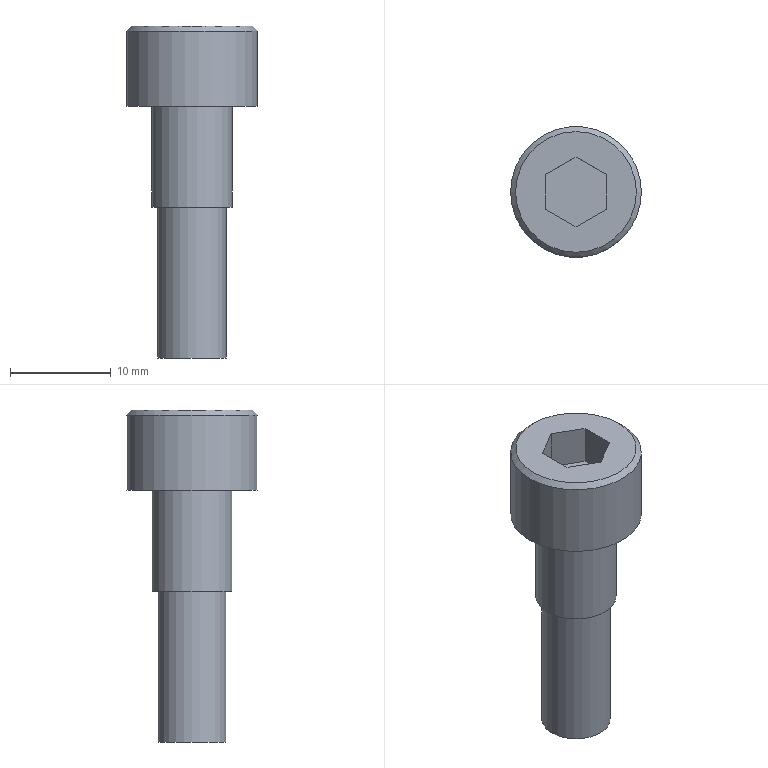Part | STEP file | M3-10_id62_x_t | 1 solid | 15 faces | box 13 x 13 x 33 mm | volume 1980 mm3 | plane 11 | cylinder 3 | cone 1 | commonest cylinder face diameters 6.8 x1 8 x1 13 x1
STEP:
#1=CARTESIAN_POINT('',(-245.9,-73.,-57.));
#2=VERTEX_POINT('',#1);
#3=CARTESIAN_POINT('',(-242.5,-73.,-57.));
#4=DIRECTION('',(0.,0.,-1.));
#5=DIRECTION('',(-1.,0.,0.));
#6=AXIS2_PLACEMENT_3D('',#3,#4,#5);
#7=CIRCLE('',#6,3.4);
#8=EDGE_CURVE('',#2,#2,#7,.T.);
#9=ORIENTED_EDGE('',*,*,#8,.F.);
#10=EDGE_LOOP('',(#9));
#11=FACE_BOUND('',#10,.T.);
#12=CARTESIAN_POINT('',(-238.5,-73.,-57.));
#13=VERTEX_POINT('',#12);
#14=CARTESIAN_POINT('',(-242.5,-73.,-57.));
#15=DIRECTION('',(0.,0.,1.));
#16=DIRECTION('',(1.,0.,0.));
#17=AXIS2_PLACEMENT_3D('',#14,#15,#16);
#18=CIRCLE('',#17,4.);
#19=EDGE_CURVE('',#13,#13,#18,.T.);
#20=ORIENTED_EDGE('',*,*,#19,.F.);
#21=EDGE_LOOP('',(#20));
#22=FACE_BOUND('',#21,.T.);
#23=CARTESIAN_POINT('',(-242.5,-73.,-57.));
#24=DIRECTION('',(0.,0.,-1.));
#25=DIRECTION('',(-1.,0.,0.));
#26=AXIS2_PLACEMENT_3D('',#23,#24,#25);
#27=PLANE('',#26);
#28=ADVANCED_FACE('',(#11,#22),#27,.T.);
#29=CARTESIAN_POINT('',(-246.5,-73.,-47.));
#30=VERTEX_POINT('',#29);
#31=CARTESIAN_POINT('',(-242.5,-73.,-47.));
#32=DIRECTION('',(0.,0.,1.));
#33=DIRECTION('',(-1.,0.,0.));
#34=AXIS2_PLACEMENT_3D('',#31,#32,#33);
#35=CIRCLE('',#34,4.);
#36=EDGE_CURVE('',#30,#30,#35,.T.);
#37=ORIENTED_EDGE('',*,*,#36,.F.);
#38=EDGE_LOOP('',(#37));
#39=FACE_BOUND('',#38,.T.);
#40=ORIENTED_EDGE('',*,*,#19,.T.);
#41=EDGE_LOOP('',(#40));
#42=FACE_BOUND('',#41,.T.);
#43=CARTESIAN_POINT('',(-242.5,-73.,-57.));
#44=DIRECTION('',(0.,0.,1.));
#45=DIRECTION('',(1.,0.,0.));
#46=AXIS2_PLACEMENT_3D('',#43,#44,#45);
#47=CYLINDRICAL_SURFACE('',#46,4.);
#48=ADVANCED_FACE('',(#39,#42),#47,.T.);
#49=CARTESIAN_POINT('',(-239.1,-73.,-72.));
#50=VERTEX_POINT('',#49);
#51=CARTESIAN_POINT('',(-242.5,-73.,-72.));
#52=DIRECTION('',(0.,0.,1.));
#53=DIRECTION('',(1.,0.,0.));
#54=AXIS2_PLACEMENT_3D('',#51,#52,#53);
#55=CIRCLE('',#54,3.4);
#56=EDGE_CURVE('',#50,#50,#55,.T.);
#57=ORIENTED_EDGE('',*,*,#56,.F.);
#58=EDGE_LOOP('',(#57));
#59=FACE_OUTER_BOUND('',#58,.T.);
#60=CARTESIAN_POINT('',(-242.5,-73.,-72.));
#61=DIRECTION('',(0.,0.,-1.));
#62=DIRECTION('',(-1.,0.,0.));
#63=AXIS2_PLACEMENT_3D('',#60,#61,#62);
#64=PLANE('',#63);
#65=ADVANCED_FACE('',(#59),#64,.T.);
#66=ORIENTED_EDGE('',*,*,#56,.T.);
#67=EDGE_LOOP('',(#66));
#68=FACE_BOUND('',#67,.T.);
#69=ORIENTED_EDGE('',*,*,#8,.T.);
#70=EDGE_LOOP('',(#69));
#71=FACE_BOUND('',#70,.T.);
#72=CARTESIAN_POINT('',(-242.5,-73.,-57.));
#73=DIRECTION('',(0.,0.,-1.));
#74=DIRECTION('',(1.,0.,0.));
#75=AXIS2_PLACEMENT_3D('',#72,#73,#74);
#76=CYLINDRICAL_SURFACE('',#75,3.4);
#77=ADVANCED_FACE('',(#68,#71),#76,.T.);
#78=CARTESIAN_POINT('',(-245.5,-71.268,-39.));
#79=VERTEX_POINT('',#78);
#80=CARTESIAN_POINT('',(-245.5,-74.732,-39.));
#81=VERTEX_POINT('',#80);
#82=CARTESIAN_POINT('',(-245.5,-71.268,-39.));
#83=DIRECTION('',(0.,-1.,0.));
#84=VECTOR('',#83,1.);
#85=LINE('',#82,#84);
#86=EDGE_CURVE('',#79,#81,#85,.T.);
#87=ORIENTED_EDGE('',*,*,#86,.F.);
#88=CARTESIAN_POINT('',(-242.5,-69.536,-39.));
#89=VERTEX_POINT('',#88);
#90=CARTESIAN_POINT('',(-242.5,-69.536,-39.));
#91=DIRECTION('',(-0.866,-0.5,0.));
#92=VECTOR('',#91,1.);
#93=LINE('',#90,#92);
#94=EDGE_CURVE('',#89,#79,#93,.T.);
#95=ORIENTED_EDGE('',*,*,#94,.F.);
#96=CARTESIAN_POINT('',(-239.5,-71.268,-39.));
#97=VERTEX_POINT('',#96);
#98=CARTESIAN_POINT('',(-239.5,-71.268,-39.));
#99=DIRECTION('',(-0.866,0.5,0.));
#100=VECTOR('',#99,1.);
#101=LINE('',#98,#100);
#102=EDGE_CURVE('',#97,#89,#101,.T.);
#103=ORIENTED_EDGE('',*,*,#102,.F.);
#104=CARTESIAN_POINT('',(-239.5,-74.732,-39.));
#105=VERTEX_POINT('',#104);
#106=CARTESIAN_POINT('',(-239.5,-74.732,-39.));
#107=DIRECTION('',(0.,1.,0.));
#108=VECTOR('',#107,1.);
#109=LINE('',#106,#108);
#110=EDGE_CURVE('',#105,#97,#109,.T.);
#111=ORIENTED_EDGE('',*,*,#110,.F.);
#112=CARTESIAN_POINT('',(-242.5,-76.464,-39.));
#113=VERTEX_POINT('',#112);
#114=CARTESIAN_POINT('',(-242.5,-76.464,-39.));
#115=DIRECTION('',(0.866,0.5,0.));
#116=VECTOR('',#115,1.);
#117=LINE('',#114,#116);
#118=EDGE_CURVE('',#113,#105,#117,.T.);
#119=ORIENTED_EDGE('',*,*,#118,.F.);
#120=CARTESIAN_POINT('',(-245.5,-74.732,-39.));
#121=DIRECTION('',(0.866,-0.5,0.));
#122=VECTOR('',#121,1.);
#123=LINE('',#120,#122);
#124=EDGE_CURVE('',#81,#113,#123,.T.);
#125=ORIENTED_EDGE('',*,*,#124,.F.);
#126=EDGE_LOOP('',(#87,#95,#103,#111,#119,#125));
#127=FACE_BOUND('',#126,.T.);
#128=CARTESIAN_POINT('',(-236.5,-73.,-39.));
#129=VERTEX_POINT('',#128);
#130=CARTESIAN_POINT('',(-242.5,-73.,-39.));
#131=DIRECTION('',(0.,0.,1.));
#132=DIRECTION('',(1.,0.,0.));
#133=AXIS2_PLACEMENT_3D('',#130,#131,#132);
#134=CIRCLE('',#133,6.);
#135=EDGE_CURVE('',#129,#129,#134,.T.);
#136=ORIENTED_EDGE('',*,*,#135,.T.);
#137=EDGE_LOOP('',(#136));
#138=FACE_BOUND('',#137,.T.);
#139=CARTESIAN_POINT('',(-242.5,-73.,-39.));
#140=DIRECTION('',(0.,0.,1.));
#141=DIRECTION('',(1.,0.,0.));
#142=AXIS2_PLACEMENT_3D('',#139,#140,#141);
#143=PLANE('',#142);
#144=ADVANCED_FACE('',(#127,#138),#143,.T.);
#145=ORIENTED_EDGE('',*,*,#36,.T.);
#146=EDGE_LOOP('',(#145));
#147=FACE_BOUND('',#146,.T.);
#148=CARTESIAN_POINT('',(-236.,-73.,-47.));
#149=VERTEX_POINT('',#148);
#150=CARTESIAN_POINT('',(-242.5,-73.,-47.));
#151=DIRECTION('',(0.,0.,1.));
#152=DIRECTION('',(1.,0.,0.));
#153=AXIS2_PLACEMENT_3D('',#150,#151,#152);
#154=CIRCLE('',#153,6.5);
#155=EDGE_CURVE('',#149,#149,#154,.T.);
#156=ORIENTED_EDGE('',*,*,#155,.F.);
#157=EDGE_LOOP('',(#156));
#158=FACE_BOUND('',#157,.T.);
#159=CARTESIAN_POINT('',(-242.5,-73.,-47.));
#160=DIRECTION('',(0.,0.,-1.));
#161=DIRECTION('',(-1.,0.,0.));
#162=AXIS2_PLACEMENT_3D('',#159,#160,#161);
#163=PLANE('',#162);
#164=ADVANCED_FACE('',(#147,#158),#163,.T.);
#165=CARTESIAN_POINT('',(-236.,-73.,-39.5));
#166=VERTEX_POINT('',#165);
#167=CARTESIAN_POINT('',(-242.5,-73.,-39.5));
#168=DIRECTION('',(0.,0.,-1.));
#169=DIRECTION('',(1.,0.,0.));
#170=AXIS2_PLACEMENT_3D('',#167,#168,#169);
#171=CIRCLE('',#170,6.5);
#172=EDGE_CURVE('',#166,#166,#171,.T.);
#173=ORIENTED_EDGE('',*,*,#172,.T.);
#174=EDGE_LOOP('',(#173));
#175=FACE_BOUND('',#174,.T.);
#176=ORIENTED_EDGE('',*,*,#155,.T.);
#177=EDGE_LOOP('',(#176));
#178=FACE_BOUND('',#177,.T.);
#179=CARTESIAN_POINT('',(-242.5,-73.,-47.));
#180=DIRECTION('',(0.,0.,1.));
#181=DIRECTION('',(1.,0.,0.));
#182=AXIS2_PLACEMENT_3D('',#179,#180,#181);
#183=CYLINDRICAL_SURFACE('',#182,6.5);
#184=ADVANCED_FACE('',(#175,#178),#183,.T.);
#185=ORIENTED_EDGE('',*,*,#135,.F.);
#186=EDGE_LOOP('',(#185));
#187=FACE_BOUND('',#186,.T.);
#188=ORIENTED_EDGE('',*,*,#172,.F.);
#189=EDGE_LOOP('',(#188));
#190=FACE_BOUND('',#189,.T.);
#191=CARTESIAN_POINT('',(-242.5,-73.,-39.5));
#192=DIRECTION('',(0.,0.,-1.));
#193=DIRECTION('',(-1.,0.,0.));
#194=AXIS2_PLACEMENT_3D('',#191,#192,#193);
#195=CONICAL_SURFACE('',#194,6.5,45.);
#196=ADVANCED_FACE('',(#187,#190),#195,.T.);
#197=ORIENTED_EDGE('',*,*,#86,.T.);
#198=CARTESIAN_POINT('',(-245.5,-74.732,-43.));
#199=VERTEX_POINT('',#198);
#200=CARTESIAN_POINT('',(-245.5,-74.732,-43.));
#201=DIRECTION('',(0.,0.,-1.));
#202=VECTOR('',#201,1.);
#203=LINE('',#200,#202);
#204=EDGE_CURVE('',#81,#199,#203,.T.);
#205=ORIENTED_EDGE('',*,*,#204,.T.);
#206=CARTESIAN_POINT('',(-245.5,-71.268,-43.));
#207=VERTEX_POINT('',#206);
#208=CARTESIAN_POINT('',(-245.5,-71.268,-43.));
#209=DIRECTION('',(0.,1.,0.));
#210=VECTOR('',#209,1.);
#211=LINE('',#208,#210);
#212=EDGE_CURVE('',#199,#207,#211,.T.);
#213=ORIENTED_EDGE('',*,*,#212,.T.);
#214=CARTESIAN_POINT('',(-245.5,-71.268,-43.));
#215=DIRECTION('',(0.,0.,-1.));
#216=VECTOR('',#215,1.);
#217=LINE('',#214,#216);
#218=EDGE_CURVE('',#79,#207,#217,.T.);
#219=ORIENTED_EDGE('',*,*,#218,.F.);
#220=EDGE_LOOP('',(#197,#205,#213,#219));
#221=FACE_OUTER_BOUND('',#220,.T.);
#222=CARTESIAN_POINT('',(-245.5,-71.268,-43.));
#223=DIRECTION('',(-1.,0.,0.));
#224=DIRECTION('',(0.,0.,1.));
#225=AXIS2_PLACEMENT_3D('',#222,#223,#224);
#226=PLANE('',#225);
#227=ADVANCED_FACE('',(#221),#226,.F.);
#228=ORIENTED_EDGE('',*,*,#124,.T.);
#229=CARTESIAN_POINT('',(-242.5,-76.464,-43.));
#230=VERTEX_POINT('',#229);
#231=CARTESIAN_POINT('',(-242.5,-76.464,-43.));
#232=DIRECTION('',(0.,0.,-1.));
#233=VECTOR('',#232,1.);
#234=LINE('',#231,#233);
#235=EDGE_CURVE('',#113,#230,#234,.T.);
#236=ORIENTED_EDGE('',*,*,#235,.T.);
#237=CARTESIAN_POINT('',(-245.5,-74.732,-43.));
#238=DIRECTION('',(-0.866,0.5,0.));
#239=VECTOR('',#238,1.);
#240=LINE('',#237,#239);
#241=EDGE_CURVE('',#230,#199,#240,.T.);
#242=ORIENTED_EDGE('',*,*,#241,.T.);
#243=ORIENTED_EDGE('',*,*,#204,.F.);
#244=EDGE_LOOP('',(#228,#236,#242,#243));
#245=FACE_OUTER_BOUND('',#244,.T.);
#246=CARTESIAN_POINT('',(-245.5,-74.732,-43.));
#247=DIRECTION('',(-0.5,-0.866,0.));
#248=DIRECTION('',(0.866,-0.5,0.));
#249=AXIS2_PLACEMENT_3D('',#246,#247,#248);
#250=PLANE('',#249);
#251=ADVANCED_FACE('',(#245),#250,.F.);
#252=ORIENTED_EDGE('',*,*,#118,.T.);
#253=CARTESIAN_POINT('',(-239.5,-74.732,-43.));
#254=VERTEX_POINT('',#253);
#255=CARTESIAN_POINT('',(-239.5,-74.732,-43.));
#256=DIRECTION('',(0.,0.,-1.));
#257=VECTOR('',#256,1.);
#258=LINE('',#255,#257);
#259=EDGE_CURVE('',#105,#254,#258,.T.);
#260=ORIENTED_EDGE('',*,*,#259,.T.);
#261=CARTESIAN_POINT('',(-242.5,-76.464,-43.));
#262=DIRECTION('',(-0.866,-0.5,0.));
#263=VECTOR('',#262,1.);
#264=LINE('',#261,#263);
#265=EDGE_CURVE('',#254,#230,#264,.T.);
#266=ORIENTED_EDGE('',*,*,#265,.T.);
#267=ORIENTED_EDGE('',*,*,#235,.F.);
#268=EDGE_LOOP('',(#252,#260,#266,#267));
#269=FACE_OUTER_BOUND('',#268,.T.);
#270=CARTESIAN_POINT('',(-242.5,-76.464,-43.));
#271=DIRECTION('',(0.5,-0.866,0.));
#272=DIRECTION('',(0.866,0.5,0.));
#273=AXIS2_PLACEMENT_3D('',#270,#271,#272);
#274=PLANE('',#273);
#275=ADVANCED_FACE('',(#269),#274,.F.);
#276=ORIENTED_EDGE('',*,*,#110,.T.);
#277=CARTESIAN_POINT('',(-239.5,-71.268,-43.));
#278=VERTEX_POINT('',#277);
#279=CARTESIAN_POINT('',(-239.5,-71.268,-43.));
#280=DIRECTION('',(0.,0.,-1.));
#281=VECTOR('',#280,1.);
#282=LINE('',#279,#281);
#283=EDGE_CURVE('',#97,#278,#282,.T.);
#284=ORIENTED_EDGE('',*,*,#283,.T.);
#285=CARTESIAN_POINT('',(-239.5,-74.732,-43.));
#286=DIRECTION('',(0.,-1.,0.));
#287=VECTOR('',#286,1.);
#288=LINE('',#285,#287);
#289=EDGE_CURVE('',#278,#254,#288,.T.);
#290=ORIENTED_EDGE('',*,*,#289,.T.);
#291=ORIENTED_EDGE('',*,*,#259,.F.);
#292=EDGE_LOOP('',(#276,#284,#290,#291));
#293=FACE_OUTER_BOUND('',#292,.T.);
#294=CARTESIAN_POINT('',(-239.5,-74.732,-43.));
#295=DIRECTION('',(1.,0.,0.));
#296=DIRECTION('',(0.,1.,0.));
#297=AXIS2_PLACEMENT_3D('',#294,#295,#296);
#298=PLANE('',#297);
#299=ADVANCED_FACE('',(#293),#298,.F.);
#300=ORIENTED_EDGE('',*,*,#102,.T.);
#301=CARTESIAN_POINT('',(-242.5,-69.536,-43.));
#302=VERTEX_POINT('',#301);
#303=CARTESIAN_POINT('',(-242.5,-69.536,-43.));
#304=DIRECTION('',(0.,0.,-1.));
#305=VECTOR('',#304,1.);
#306=LINE('',#303,#305);
#307=EDGE_CURVE('',#89,#302,#306,.T.);
#308=ORIENTED_EDGE('',*,*,#307,.T.);
#309=CARTESIAN_POINT('',(-239.5,-71.268,-43.));
#310=DIRECTION('',(0.866,-0.5,0.));
#311=VECTOR('',#310,1.);
#312=LINE('',#309,#311);
#313=EDGE_CURVE('',#302,#278,#312,.T.);
#314=ORIENTED_EDGE('',*,*,#313,.T.);
#315=ORIENTED_EDGE('',*,*,#283,.F.);
#316=EDGE_LOOP('',(#300,#308,#314,#315));
#317=FACE_OUTER_BOUND('',#316,.T.);
#318=CARTESIAN_POINT('',(-239.5,-71.268,-43.));
#319=DIRECTION('',(0.5,0.866,0.));
#320=DIRECTION('',(-0.866,0.5,0.));
#321=AXIS2_PLACEMENT_3D('',#318,#319,#320);
#322=PLANE('',#321);
#323=ADVANCED_FACE('',(#317),#322,.F.);
#324=ORIENTED_EDGE('',*,*,#94,.T.);
#325=ORIENTED_EDGE('',*,*,#218,.T.);
#326=CARTESIAN_POINT('',(-242.5,-69.536,-43.));
#327=DIRECTION('',(0.866,0.5,0.));
#328=VECTOR('',#327,1.);
#329=LINE('',#326,#328);
#330=EDGE_CURVE('',#207,#302,#329,.T.);
#331=ORIENTED_EDGE('',*,*,#330,.T.);
#332=ORIENTED_EDGE('',*,*,#307,.F.);
#333=EDGE_LOOP('',(#324,#325,#331,#332));
#334=FACE_OUTER_BOUND('',#333,.T.);
#335=CARTESIAN_POINT('',(-242.5,-69.536,-43.));
#336=DIRECTION('',(-0.5,0.866,0.));
#337=DIRECTION('',(-0.866,-0.5,0.));
#338=AXIS2_PLACEMENT_3D('',#335,#336,#337);
#339=PLANE('',#338);
#340=ADVANCED_FACE('',(#334),#339,.F.);
#341=ORIENTED_EDGE('',*,*,#212,.F.);
#342=ORIENTED_EDGE('',*,*,#241,.F.);
#343=ORIENTED_EDGE('',*,*,#265,.F.);
#344=ORIENTED_EDGE('',*,*,#289,.F.);
#345=ORIENTED_EDGE('',*,*,#313,.F.);
#346=ORIENTED_EDGE('',*,*,#330,.F.);
#347=EDGE_LOOP('',(#341,#342,#343,#344,#345,#346));
#348=FACE_OUTER_BOUND('',#347,.T.);
#349=CARTESIAN_POINT('',(-242.5,-73.,-43.));
#350=DIRECTION('',(0.,0.,1.));
#351=DIRECTION('',(1.,0.,0.));
#352=AXIS2_PLACEMENT_3D('',#349,#350,#351);
#353=PLANE('',#352);
#354=ADVANCED_FACE('',(#348),#353,.T.);
#355=CLOSED_SHELL('',(#28,#48,#65,#77,#144,#164,#184,#196,#227,#251,#275,#299,#323,#340,#354));
#356=MANIFOLD_SOLID_BREP('',#355);
#357=(LENGTH_UNIT()NAMED_UNIT(*)SI_UNIT(.MILLI.,.METRE.));
#358=UNCERTAINTY_MEASURE_WITH_UNIT(LENGTH_MEASURE(0.00002),#357,'','');
#359=(NAMED_UNIT(*)PLANE_ANGLE_UNIT()SI_UNIT($,.RADIAN.));
#360=PLANE_ANGLE_MEASURE_WITH_UNIT(PLANE_ANGLE_MEASURE(0.01745),#359);
#361=DIMENSIONAL_EXPONENTS(0.,0.,0.,0.,0.,0.,0.);
#362=(CONVERSION_BASED_UNIT('DEGREE',#360)NAMED_UNIT(#361)PLANE_ANGLE_UNIT());
#363=(NAMED_UNIT(*)SI_UNIT($,.STERADIAN.)SOLID_ANGLE_UNIT());
#364=(GEOMETRIC_REPRESENTATION_CONTEXT(3)GLOBAL_UNCERTAINTY_ASSIGNED_CONTEXT((#358))GLOBAL_UNIT_ASSIGNED_CONTEXT((#357,#362,#363))REPRESENTATION_CONTEXT('',''));
#365=ADVANCED_BREP_SHAPE_REPRESENTATION('',(#356),#364);